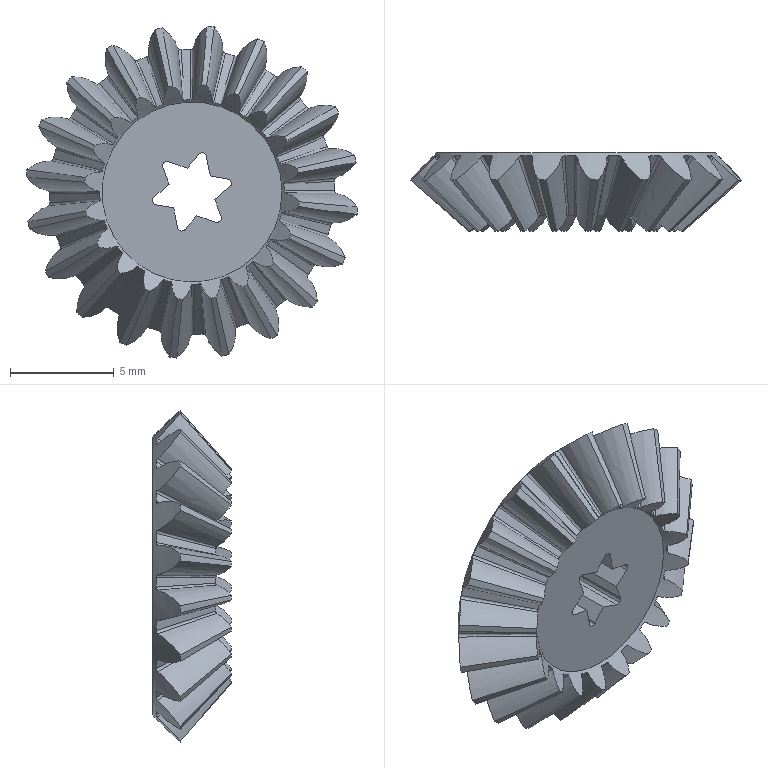Part | STEP file | Wytnij-wyci_gni_cie2_1 | 1 solid | 144 faces | box 15.995 x 3.782 x 15.995 mm | volume 380.18 mm3 | spline 108 | cone 14 | plane 14 | cylinder 8 | commonest cylinder face diameters 0.42 x8